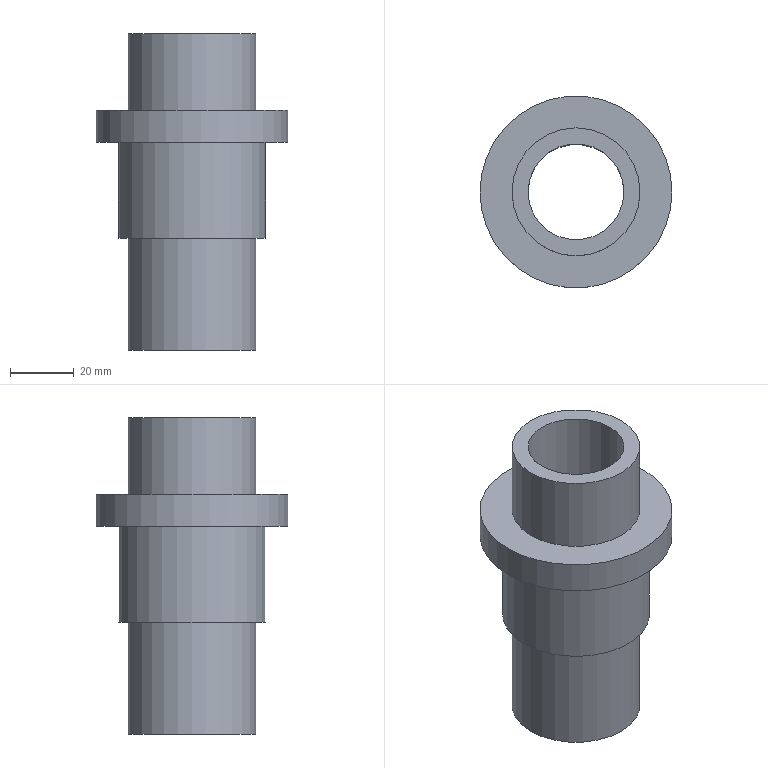Part | NX | features solid 2 | 1 solid | 10 faces | box 60 x 60 x 99 mm | volume 82294 mm3 | cylinder 5 | plane 5 | commonest cylinder face diameters 40 x2 30 x1 46 x1 60 x1
STEP:
#1=CARTESIAN_POINT('',(-47.,-155.,-190.));
#2=VERTEX_POINT('',#1);
#3=CARTESIAN_POINT('',(-70.,-155.,-190.));
#4=DIRECTION('',(0.,0.,1.));
#5=DIRECTION('',(1.,0.,0.));
#6=AXIS2_PLACEMENT_3D('',#3,#4,#5);
#7=CIRCLE('',#6,23.);
#8=EDGE_CURVE('',#2,#2,#7,.T.);
#9=ORIENTED_EDGE('',*,*,#8,.T.);
#10=EDGE_LOOP('',(#9));
#11=FACE_BOUND('',#10,.T.);
#12=CARTESIAN_POINT('',(-47.,-155.,-160.));
#13=VERTEX_POINT('',#12);
#14=CARTESIAN_POINT('',(-70.,-155.,-160.));
#15=DIRECTION('',(0.,0.,1.));
#16=DIRECTION('',(1.,0.,0.));
#17=AXIS2_PLACEMENT_3D('',#14,#15,#16);
#18=CIRCLE('',#17,23.);
#19=EDGE_CURVE('',#13,#13,#18,.T.);
#20=ORIENTED_EDGE('',*,*,#19,.F.);
#21=EDGE_LOOP('',(#20));
#22=FACE_BOUND('',#21,.T.);
#23=CARTESIAN_POINT('',(-70.,-155.,-150.));
#24=DIRECTION('',(0.,0.,-1.));
#25=DIRECTION('',(-1.,0.,0.));
#26=AXIS2_PLACEMENT_3D('',#23,#24,#25);
#27=CYLINDRICAL_SURFACE('',#26,23.);
#28=ADVANCED_FACE('',(#11,#22),#27,.T.);
#29=CARTESIAN_POINT('',(-50.,-155.,-225.));
#30=VERTEX_POINT('',#29);
#31=CARTESIAN_POINT('',(-70.,-155.,-225.));
#32=DIRECTION('',(0.,0.,1.));
#33=DIRECTION('',(1.,0.,0.));
#34=AXIS2_PLACEMENT_3D('',#31,#32,#33);
#35=CIRCLE('',#34,20.);
#36=EDGE_CURVE('',#30,#30,#35,.T.);
#37=ORIENTED_EDGE('',*,*,#36,.T.);
#38=EDGE_LOOP('',(#37));
#39=FACE_BOUND('',#38,.T.);
#40=CARTESIAN_POINT('',(-50.,-155.,-190.));
#41=VERTEX_POINT('',#40);
#42=CARTESIAN_POINT('',(-70.,-155.,-190.));
#43=DIRECTION('',(0.,0.,1.));
#44=DIRECTION('',(1.,0.,0.));
#45=AXIS2_PLACEMENT_3D('',#42,#43,#44);
#46=CIRCLE('',#45,20.);
#47=EDGE_CURVE('',#41,#41,#46,.T.);
#48=ORIENTED_EDGE('',*,*,#47,.F.);
#49=EDGE_LOOP('',(#48));
#50=FACE_BOUND('',#49,.T.);
#51=CARTESIAN_POINT('',(-70.,-155.,-126.));
#52=DIRECTION('',(0.,0.,-1.));
#53=DIRECTION('',(-1.,0.,0.));
#54=AXIS2_PLACEMENT_3D('',#51,#52,#53);
#55=CYLINDRICAL_SURFACE('',#54,20.);
#56=ADVANCED_FACE('',(#39,#50),#55,.T.);
#57=CARTESIAN_POINT('',(-55.,-155.,-126.));
#58=VERTEX_POINT('',#57);
#59=CARTESIAN_POINT('',(-70.,-155.,-126.));
#60=DIRECTION('',(0.,0.,1.));
#61=DIRECTION('',(1.,0.,0.));
#62=AXIS2_PLACEMENT_3D('',#59,#60,#61);
#63=CIRCLE('',#62,15.);
#64=EDGE_CURVE('',#58,#58,#63,.T.);
#65=ORIENTED_EDGE('',*,*,#64,.T.);
#66=EDGE_LOOP('',(#65));
#67=FACE_BOUND('',#66,.T.);
#68=CARTESIAN_POINT('',(-55.,-155.,-225.));
#69=VERTEX_POINT('',#68);
#70=CARTESIAN_POINT('',(-70.,-155.,-225.));
#71=DIRECTION('',(0.,0.,1.));
#72=DIRECTION('',(1.,0.,0.));
#73=AXIS2_PLACEMENT_3D('',#70,#71,#72);
#74=CIRCLE('',#73,15.);
#75=EDGE_CURVE('',#69,#69,#74,.T.);
#76=ORIENTED_EDGE('',*,*,#75,.F.);
#77=EDGE_LOOP('',(#76));
#78=FACE_BOUND('',#77,.T.);
#79=CARTESIAN_POINT('',(-70.,-155.,-126.));
#80=DIRECTION('',(0.,0.,-1.));
#81=DIRECTION('',(-1.,0.,0.));
#82=AXIS2_PLACEMENT_3D('',#79,#80,#81);
#83=CYLINDRICAL_SURFACE('',#82,15.);
#84=ADVANCED_FACE('',(#67,#78),#83,.F.);
#85=CARTESIAN_POINT('',(-50.,-155.,-150.));
#86=VERTEX_POINT('',#85);
#87=CARTESIAN_POINT('',(-70.,-155.,-150.));
#88=DIRECTION('',(0.,0.,1.));
#89=DIRECTION('',(1.,0.,0.));
#90=AXIS2_PLACEMENT_3D('',#87,#88,#89);
#91=CIRCLE('',#90,20.);
#92=EDGE_CURVE('',#86,#86,#91,.T.);
#93=ORIENTED_EDGE('',*,*,#92,.T.);
#94=EDGE_LOOP('',(#93));
#95=FACE_BOUND('',#94,.T.);
#96=CARTESIAN_POINT('',(-50.,-155.,-126.));
#97=VERTEX_POINT('',#96);
#98=CARTESIAN_POINT('',(-70.,-155.,-126.));
#99=DIRECTION('',(0.,0.,1.));
#100=DIRECTION('',(1.,0.,0.));
#101=AXIS2_PLACEMENT_3D('',#98,#99,#100);
#102=CIRCLE('',#101,20.);
#103=EDGE_CURVE('',#97,#97,#102,.T.);
#104=ORIENTED_EDGE('',*,*,#103,.F.);
#105=EDGE_LOOP('',(#104));
#106=FACE_BOUND('',#105,.T.);
#107=CARTESIAN_POINT('',(-70.,-155.,-126.));
#108=DIRECTION('',(0.,0.,-1.));
#109=DIRECTION('',(-1.,0.,0.));
#110=AXIS2_PLACEMENT_3D('',#107,#108,#109);
#111=CYLINDRICAL_SURFACE('',#110,20.);
#112=ADVANCED_FACE('',(#95,#106),#111,.T.);
#113=ORIENTED_EDGE('',*,*,#64,.F.);
#114=EDGE_LOOP('',(#113));
#115=FACE_BOUND('',#114,.T.);
#116=ORIENTED_EDGE('',*,*,#103,.T.);
#117=EDGE_LOOP('',(#116));
#118=FACE_BOUND('',#117,.T.);
#119=CARTESIAN_POINT('',(-70.,-155.,-126.));
#120=DIRECTION('',(0.,0.,1.));
#121=DIRECTION('',(1.,0.,0.));
#122=AXIS2_PLACEMENT_3D('',#119,#120,#121);
#123=PLANE('',#122);
#124=ADVANCED_FACE('',(#115,#118),#123,.T.);
#125=ORIENTED_EDGE('',*,*,#75,.T.);
#126=EDGE_LOOP('',(#125));
#127=FACE_BOUND('',#126,.T.);
#128=ORIENTED_EDGE('',*,*,#36,.F.);
#129=EDGE_LOOP('',(#128));
#130=FACE_BOUND('',#129,.T.);
#131=CARTESIAN_POINT('',(-70.,-155.,-225.));
#132=DIRECTION('',(0.,0.,1.));
#133=DIRECTION('',(1.,0.,0.));
#134=AXIS2_PLACEMENT_3D('',#131,#132,#133);
#135=PLANE('',#134);
#136=ADVANCED_FACE('',(#127,#130),#135,.F.);
#137=ORIENTED_EDGE('',*,*,#92,.F.);
#138=EDGE_LOOP('',(#137));
#139=FACE_BOUND('',#138,.T.);
#140=CARTESIAN_POINT('',(-40.,-155.,-150.));
#141=VERTEX_POINT('',#140);
#142=CARTESIAN_POINT('',(-70.,-155.,-150.));
#143=DIRECTION('',(0.,0.,1.));
#144=DIRECTION('',(1.,0.,0.));
#145=AXIS2_PLACEMENT_3D('',#142,#143,#144);
#146=CIRCLE('',#145,30.);
#147=EDGE_CURVE('',#141,#141,#146,.T.);
#148=ORIENTED_EDGE('',*,*,#147,.T.);
#149=EDGE_LOOP('',(#148));
#150=FACE_BOUND('',#149,.T.);
#151=CARTESIAN_POINT('',(-70.,-155.,-150.));
#152=DIRECTION('',(0.,0.,1.));
#153=DIRECTION('',(1.,0.,0.));
#154=AXIS2_PLACEMENT_3D('',#151,#152,#153);
#155=PLANE('',#154);
#156=ADVANCED_FACE('',(#139,#150),#155,.T.);
#157=ORIENTED_EDGE('',*,*,#47,.T.);
#158=EDGE_LOOP('',(#157));
#159=FACE_BOUND('',#158,.T.);
#160=ORIENTED_EDGE('',*,*,#8,.F.);
#161=EDGE_LOOP('',(#160));
#162=FACE_BOUND('',#161,.T.);
#163=CARTESIAN_POINT('',(-70.,-155.,-190.));
#164=DIRECTION('',(0.,0.,1.));
#165=DIRECTION('',(1.,0.,0.));
#166=AXIS2_PLACEMENT_3D('',#163,#164,#165);
#167=PLANE('',#166);
#168=ADVANCED_FACE('',(#159,#162),#167,.F.);
#169=CARTESIAN_POINT('',(-40.,-155.,-160.));
#170=VERTEX_POINT('',#169);
#171=CARTESIAN_POINT('',(-70.,-155.,-160.));
#172=DIRECTION('',(0.,0.,1.));
#173=DIRECTION('',(1.,0.,0.));
#174=AXIS2_PLACEMENT_3D('',#171,#172,#173);
#175=CIRCLE('',#174,30.);
#176=EDGE_CURVE('',#170,#170,#175,.T.);
#177=ORIENTED_EDGE('',*,*,#176,.F.);
#178=EDGE_LOOP('',(#177));
#179=FACE_BOUND('',#178,.T.);
#180=ORIENTED_EDGE('',*,*,#19,.T.);
#181=EDGE_LOOP('',(#180));
#182=FACE_BOUND('',#181,.T.);
#183=CARTESIAN_POINT('',(-70.,-155.,-160.));
#184=DIRECTION('',(0.,0.,1.));
#185=DIRECTION('',(1.,0.,0.));
#186=AXIS2_PLACEMENT_3D('',#183,#184,#185);
#187=PLANE('',#186);
#188=ADVANCED_FACE('',(#179,#182),#187,.F.);
#189=ORIENTED_EDGE('',*,*,#147,.F.);
#190=EDGE_LOOP('',(#189));
#191=FACE_BOUND('',#190,.T.);
#192=ORIENTED_EDGE('',*,*,#176,.T.);
#193=EDGE_LOOP('',(#192));
#194=FACE_BOUND('',#193,.T.);
#195=CARTESIAN_POINT('',(-70.,-155.,-150.));
#196=DIRECTION('',(0.,0.,-1.));
#197=DIRECTION('',(-1.,0.,0.));
#198=AXIS2_PLACEMENT_3D('',#195,#196,#197);
#199=CYLINDRICAL_SURFACE('',#198,30.);
#200=ADVANCED_FACE('',(#191,#194),#199,.T.);
#201=CLOSED_SHELL('',(#28,#56,#84,#112,#124,#136,#156,#168,#188,#200));
#202=MANIFOLD_SOLID_BREP('',#201);
#203=(LENGTH_UNIT()NAMED_UNIT(*)SI_UNIT(.MILLI.,.METRE.));
#204=UNCERTAINTY_MEASURE_WITH_UNIT(LENGTH_MEASURE(0.00001),#203,'','');
#205=(NAMED_UNIT(*)PLANE_ANGLE_UNIT()SI_UNIT($,.RADIAN.));
#206=(NAMED_UNIT(*)SI_UNIT($,.STERADIAN.)SOLID_ANGLE_UNIT());
#207=(GEOMETRIC_REPRESENTATION_CONTEXT(3)GLOBAL_UNCERTAINTY_ASSIGNED_CONTEXT((#204))GLOBAL_UNIT_ASSIGNED_CONTEXT((#203,#205,#206))REPRESENTATION_CONTEXT('',''));
#208=ADVANCED_BREP_SHAPE_REPRESENTATION('',(#202),#207);